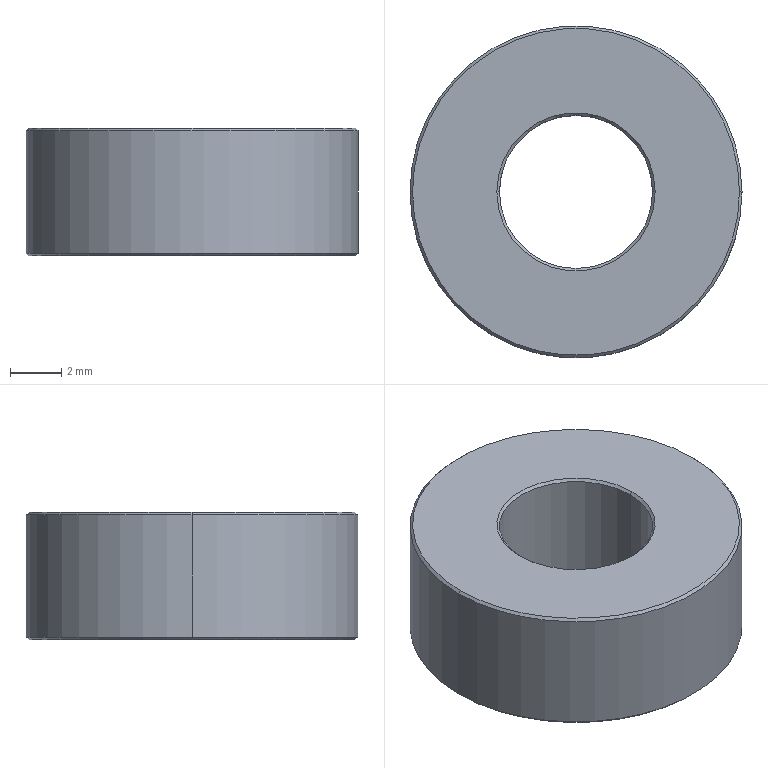Part | SolidWorks | features Chamfer 1, Extrusion 1 | 1 solid | 14 faces | box 13 x 13 x 5 mm | volume 521.693 mm3 | cone 8 | cylinder 4 | plane 2 | commonest cylinder face diameters 6 x2 13 x2
STEP:
#1=CARTESIAN_POINT('',(-6.4,0.,0.));
#2=VERTEX_POINT('',#1);
#3=CARTESIAN_POINT('',(6.4,0.,0.));
#4=VERTEX_POINT('',#3);
#5=CARTESIAN_POINT('',(0.,0.,0.));
#6=DIRECTION('',(0.,0.,-1.));
#7=DIRECTION('',(1.,0.,0.));
#8=AXIS2_PLACEMENT_3D('',#5,#6,#7);
#9=CIRCLE('',#8,6.4);
#10=EDGE_CURVE('',#2,#4,#9,.T.);
#11=ORIENTED_EDGE('',*,*,#10,.F.);
#12=CARTESIAN_POINT('',(-6.5,0.,0.1));
#13=VERTEX_POINT('',#12);
#14=CARTESIAN_POINT('',(-6.5,0.,0.1));
#15=DIRECTION('',(-0.7071,0.,0.7071));
#16=VECTOR('',#15,1000.);
#17=LINE('',#14,#16);
#18=EDGE_CURVE('',#2,#13,#17,.T.);
#19=ORIENTED_EDGE('',*,*,#18,.T.);
#20=CARTESIAN_POINT('',(6.5,0.,0.1));
#21=VERTEX_POINT('',#20);
#22=CARTESIAN_POINT('',(0.,0.,0.1));
#23=DIRECTION('',(0.,0.,1.));
#24=DIRECTION('',(1.,0.,0.));
#25=AXIS2_PLACEMENT_3D('',#22,#23,#24);
#26=CIRCLE('',#25,6.5);
#27=EDGE_CURVE('',#21,#13,#26,.T.);
#28=ORIENTED_EDGE('',*,*,#27,.F.);
#29=CARTESIAN_POINT('',(6.5,0.,0.1));
#30=DIRECTION('',(0.7071,0.,0.7071));
#31=VECTOR('',#30,1000.);
#32=LINE('',#29,#31);
#33=EDGE_CURVE('',#4,#21,#32,.T.);
#34=ORIENTED_EDGE('',*,*,#33,.F.);
#35=EDGE_LOOP('',(#11,#19,#28,#34));
#36=FACE_OUTER_BOUND('',#35,.T.);
#37=CARTESIAN_POINT('',(0.,0.,0.1));
#38=DIRECTION('',(0.,0.,1.));
#39=DIRECTION('',(1.,0.,0.));
#40=AXIS2_PLACEMENT_3D('',#37,#38,#39);
#41=CONICAL_SURFACE('',#40,6.5,0.7854);
#42=ADVANCED_FACE('',(#36),#41,.T.);
#43=CARTESIAN_POINT('',(3.,0.,0.1));
#44=VERTEX_POINT('',#43);
#45=CARTESIAN_POINT('',(-3.,0.,0.1));
#46=VERTEX_POINT('',#45);
#47=CARTESIAN_POINT('',(0.,0.,0.1));
#48=DIRECTION('',(0.,0.,-1.));
#49=DIRECTION('',(1.,0.,0.));
#50=AXIS2_PLACEMENT_3D('',#47,#48,#49);
#51=CIRCLE('',#50,3.);
#52=EDGE_CURVE('',#44,#46,#51,.T.);
#53=ORIENTED_EDGE('',*,*,#52,.F.);
#54=CARTESIAN_POINT('',(3.1,0.,0.));
#55=VERTEX_POINT('',#54);
#56=CARTESIAN_POINT('',(3.1,0.,0.));
#57=DIRECTION('',(0.7071,0.,-0.7071));
#58=VECTOR('',#57,1000.);
#59=LINE('',#56,#58);
#60=EDGE_CURVE('',#44,#55,#59,.T.);
#61=ORIENTED_EDGE('',*,*,#60,.T.);
#62=CARTESIAN_POINT('',(-3.1,0.,0.));
#63=VERTEX_POINT('',#62);
#64=CARTESIAN_POINT('',(0.,0.,0.));
#65=DIRECTION('',(0.,0.,1.));
#66=DIRECTION('',(1.,0.,0.));
#67=AXIS2_PLACEMENT_3D('',#64,#65,#66);
#68=CIRCLE('',#67,3.1);
#69=EDGE_CURVE('',#63,#55,#68,.T.);
#70=ORIENTED_EDGE('',*,*,#69,.F.);
#71=CARTESIAN_POINT('',(-3.1,0.,0.));
#72=DIRECTION('',(-0.7071,0.,-0.7071));
#73=VECTOR('',#72,1000.);
#74=LINE('',#71,#73);
#75=EDGE_CURVE('',#46,#63,#74,.T.);
#76=ORIENTED_EDGE('',*,*,#75,.F.);
#77=EDGE_LOOP('',(#53,#61,#70,#76));
#78=FACE_OUTER_BOUND('',#77,.T.);
#79=CARTESIAN_POINT('',(0.,0.,0.));
#80=DIRECTION('',(0.,0.,-1.));
#81=DIRECTION('',(-1.,0.,0.));
#82=AXIS2_PLACEMENT_3D('',#79,#80,#81);
#83=CONICAL_SURFACE('',#82,3.1,0.7854);
#84=ADVANCED_FACE('',(#78),#83,.F.);
#85=CARTESIAN_POINT('',(6.4,0.,5.));
#86=VERTEX_POINT('',#85);
#87=CARTESIAN_POINT('',(-6.4,0.,5.));
#88=VERTEX_POINT('',#87);
#89=CARTESIAN_POINT('',(0.,0.,5.));
#90=DIRECTION('',(0.,0.,1.));
#91=DIRECTION('',(1.,0.,0.));
#92=AXIS2_PLACEMENT_3D('',#89,#90,#91);
#93=CIRCLE('',#92,6.4);
#94=EDGE_CURVE('',#86,#88,#93,.T.);
#95=ORIENTED_EDGE('',*,*,#94,.F.);
#96=CARTESIAN_POINT('',(6.5,0.,4.9));
#97=VERTEX_POINT('',#96);
#98=CARTESIAN_POINT('',(6.4,0.,5.));
#99=DIRECTION('',(0.7071,0.,-0.7071));
#100=VECTOR('',#99,1000.);
#101=LINE('',#98,#100);
#102=EDGE_CURVE('',#86,#97,#101,.T.);
#103=ORIENTED_EDGE('',*,*,#102,.T.);
#104=CARTESIAN_POINT('',(-6.5,0.,4.9));
#105=VERTEX_POINT('',#104);
#106=CARTESIAN_POINT('',(0.,0.,4.9));
#107=DIRECTION('',(0.,0.,-1.));
#108=DIRECTION('',(1.,0.,0.));
#109=AXIS2_PLACEMENT_3D('',#106,#107,#108);
#110=CIRCLE('',#109,6.5);
#111=EDGE_CURVE('',#105,#97,#110,.T.);
#112=ORIENTED_EDGE('',*,*,#111,.F.);
#113=CARTESIAN_POINT('',(-6.4,0.,5.));
#114=DIRECTION('',(-0.7071,0.,-0.7071));
#115=VECTOR('',#114,1000.);
#116=LINE('',#113,#115);
#117=EDGE_CURVE('',#88,#105,#116,.T.);
#118=ORIENTED_EDGE('',*,*,#117,.F.);
#119=EDGE_LOOP('',(#95,#103,#112,#118));
#120=FACE_OUTER_BOUND('',#119,.T.);
#121=CARTESIAN_POINT('',(0.,0.,5.));
#122=DIRECTION('',(0.,0.,-1.));
#123=DIRECTION('',(-1.,0.,0.));
#124=AXIS2_PLACEMENT_3D('',#121,#122,#123);
#125=CONICAL_SURFACE('',#124,6.4,0.7854);
#126=ADVANCED_FACE('',(#120),#125,.T.);
#127=CARTESIAN_POINT('',(-3.,0.,4.9));
#128=VERTEX_POINT('',#127);
#129=CARTESIAN_POINT('',(3.,0.,4.9));
#130=VERTEX_POINT('',#129);
#131=CARTESIAN_POINT('',(0.,0.,4.9));
#132=DIRECTION('',(0.,0.,1.));
#133=DIRECTION('',(1.,0.,0.));
#134=AXIS2_PLACEMENT_3D('',#131,#132,#133);
#135=CIRCLE('',#134,3.);
#136=EDGE_CURVE('',#128,#130,#135,.T.);
#137=ORIENTED_EDGE('',*,*,#136,.F.);
#138=CARTESIAN_POINT('',(-3.1,0.,5.));
#139=VERTEX_POINT('',#138);
#140=CARTESIAN_POINT('',(-3.,0.,4.9));
#141=DIRECTION('',(-0.7071,0.,0.7071));
#142=VECTOR('',#141,1000.);
#143=LINE('',#140,#142);
#144=EDGE_CURVE('',#128,#139,#143,.T.);
#145=ORIENTED_EDGE('',*,*,#144,.T.);
#146=CARTESIAN_POINT('',(3.1,0.,5.));
#147=VERTEX_POINT('',#146);
#148=CARTESIAN_POINT('',(0.,0.,5.));
#149=DIRECTION('',(0.,0.,-1.));
#150=DIRECTION('',(1.,0.,0.));
#151=AXIS2_PLACEMENT_3D('',#148,#149,#150);
#152=CIRCLE('',#151,3.1);
#153=EDGE_CURVE('',#147,#139,#152,.T.);
#154=ORIENTED_EDGE('',*,*,#153,.F.);
#155=CARTESIAN_POINT('',(3.,0.,4.9));
#156=DIRECTION('',(0.7071,0.,0.7071));
#157=VECTOR('',#156,1000.);
#158=LINE('',#155,#157);
#159=EDGE_CURVE('',#130,#147,#158,.T.);
#160=ORIENTED_EDGE('',*,*,#159,.F.);
#161=EDGE_LOOP('',(#137,#145,#154,#160));
#162=FACE_OUTER_BOUND('',#161,.T.);
#163=CARTESIAN_POINT('',(0.,0.,4.9));
#164=DIRECTION('',(0.,0.,1.));
#165=DIRECTION('',(1.,0.,0.));
#166=AXIS2_PLACEMENT_3D('',#163,#164,#165);
#167=CONICAL_SURFACE('',#166,3.,0.7854);
#168=ADVANCED_FACE('',(#162),#167,.F.);
#169=ORIENTED_EDGE('',*,*,#136,.T.);
#170=CARTESIAN_POINT('',(3.,0.,5.));
#171=DIRECTION('',(0.,0.,-1.));
#172=VECTOR('',#171,1000.);
#173=LINE('',#170,#172);
#174=EDGE_CURVE('',#130,#44,#173,.T.);
#175=ORIENTED_EDGE('',*,*,#174,.T.);
#176=ORIENTED_EDGE('',*,*,#52,.T.);
#177=CARTESIAN_POINT('',(-3.,0.,5.));
#178=DIRECTION('',(0.,0.,-1.));
#179=VECTOR('',#178,1000.);
#180=LINE('',#177,#179);
#181=EDGE_CURVE('',#128,#46,#180,.T.);
#182=ORIENTED_EDGE('',*,*,#181,.F.);
#183=EDGE_LOOP('',(#169,#175,#176,#182));
#184=FACE_OUTER_BOUND('',#183,.T.);
#185=CARTESIAN_POINT('',(0.,0.,5.));
#186=DIRECTION('',(0.,0.,-1.));
#187=DIRECTION('',(-1.,0.,0.));
#188=AXIS2_PLACEMENT_3D('',#185,#186,#187);
#189=CYLINDRICAL_SURFACE('',#188,3.);
#190=ADVANCED_FACE('',(#184),#189,.F.);
#191=ORIENTED_EDGE('',*,*,#111,.T.);
#192=CARTESIAN_POINT('',(6.5,0.,5.));
#193=DIRECTION('',(0.,0.,-1.));
#194=VECTOR('',#193,1000.);
#195=LINE('',#192,#194);
#196=EDGE_CURVE('',#97,#21,#195,.T.);
#197=ORIENTED_EDGE('',*,*,#196,.T.);
#198=ORIENTED_EDGE('',*,*,#27,.T.);
#199=CARTESIAN_POINT('',(-6.5,0.,5.));
#200=DIRECTION('',(0.,0.,-1.));
#201=VECTOR('',#200,1000.);
#202=LINE('',#199,#201);
#203=EDGE_CURVE('',#105,#13,#202,.T.);
#204=ORIENTED_EDGE('',*,*,#203,.F.);
#205=EDGE_LOOP('',(#191,#197,#198,#204));
#206=FACE_OUTER_BOUND('',#205,.T.);
#207=CARTESIAN_POINT('',(0.,0.,5.));
#208=DIRECTION('',(0.,0.,-1.));
#209=DIRECTION('',(-1.,0.,0.));
#210=AXIS2_PLACEMENT_3D('',#207,#208,#209);
#211=CYLINDRICAL_SURFACE('',#210,6.5);
#212=ADVANCED_FACE('',(#206),#211,.T.);
#213=ORIENTED_EDGE('',*,*,#153,.T.);
#214=CARTESIAN_POINT('',(0.,0.,5.));
#215=DIRECTION('',(0.,0.,-1.));
#216=DIRECTION('',(1.,0.,0.));
#217=AXIS2_PLACEMENT_3D('',#214,#215,#216);
#218=CIRCLE('',#217,3.1);
#219=EDGE_CURVE('',#139,#147,#218,.T.);
#220=ORIENTED_EDGE('',*,*,#219,.T.);
#221=EDGE_LOOP('',(#213,#220));
#222=FACE_BOUND('',#221,.T.);
#223=CARTESIAN_POINT('',(0.,0.,5.));
#224=DIRECTION('',(0.,0.,1.));
#225=DIRECTION('',(1.,0.,0.));
#226=AXIS2_PLACEMENT_3D('',#223,#224,#225);
#227=CIRCLE('',#226,6.4);
#228=EDGE_CURVE('',#88,#86,#227,.T.);
#229=ORIENTED_EDGE('',*,*,#228,.T.);
#230=ORIENTED_EDGE('',*,*,#94,.T.);
#231=EDGE_LOOP('',(#229,#230));
#232=FACE_OUTER_BOUND('',#231,.T.);
#233=CARTESIAN_POINT('',(0.,0.,5.));
#234=DIRECTION('',(0.,0.,1.));
#235=DIRECTION('',(1.,0.,0.));
#236=AXIS2_PLACEMENT_3D('',#233,#234,#235);
#237=PLANE('',#236);
#238=ADVANCED_FACE('',(#222,#232),#237,.T.);
#239=ORIENTED_EDGE('',*,*,#69,.T.);
#240=CARTESIAN_POINT('',(0.,0.,0.));
#241=DIRECTION('',(0.,0.,1.));
#242=DIRECTION('',(1.,0.,0.));
#243=AXIS2_PLACEMENT_3D('',#240,#241,#242);
#244=CIRCLE('',#243,3.1);
#245=EDGE_CURVE('',#55,#63,#244,.T.);
#246=ORIENTED_EDGE('',*,*,#245,.T.);
#247=EDGE_LOOP('',(#239,#246));
#248=FACE_BOUND('',#247,.T.);
#249=CARTESIAN_POINT('',(0.,0.,0.));
#250=DIRECTION('',(0.,0.,-1.));
#251=DIRECTION('',(1.,0.,0.));
#252=AXIS2_PLACEMENT_3D('',#249,#250,#251);
#253=CIRCLE('',#252,6.4);
#254=EDGE_CURVE('',#4,#2,#253,.T.);
#255=ORIENTED_EDGE('',*,*,#254,.T.);
#256=ORIENTED_EDGE('',*,*,#10,.T.);
#257=EDGE_LOOP('',(#255,#256));
#258=FACE_OUTER_BOUND('',#257,.T.);
#259=CARTESIAN_POINT('',(0.,0.,0.));
#260=DIRECTION('',(0.,0.,1.));
#261=DIRECTION('',(1.,0.,0.));
#262=AXIS2_PLACEMENT_3D('',#259,#260,#261);
#263=PLANE('',#262);
#264=ADVANCED_FACE('',(#248,#258),#263,.F.);
#265=ORIENTED_EDGE('',*,*,#196,.F.);
#266=CARTESIAN_POINT('',(0.,0.,4.9));
#267=DIRECTION('',(0.,0.,-1.));
#268=DIRECTION('',(1.,0.,0.));
#269=AXIS2_PLACEMENT_3D('',#266,#267,#268);
#270=CIRCLE('',#269,6.5);
#271=EDGE_CURVE('',#97,#105,#270,.T.);
#272=ORIENTED_EDGE('',*,*,#271,.T.);
#273=ORIENTED_EDGE('',*,*,#203,.T.);
#274=CARTESIAN_POINT('',(0.,0.,0.1));
#275=DIRECTION('',(0.,0.,1.));
#276=DIRECTION('',(1.,0.,0.));
#277=AXIS2_PLACEMENT_3D('',#274,#275,#276);
#278=CIRCLE('',#277,6.5);
#279=EDGE_CURVE('',#13,#21,#278,.T.);
#280=ORIENTED_EDGE('',*,*,#279,.T.);
#281=EDGE_LOOP('',(#265,#272,#273,#280));
#282=FACE_OUTER_BOUND('',#281,.T.);
#283=CARTESIAN_POINT('',(0.,0.,5.));
#284=DIRECTION('',(0.,0.,-1.));
#285=DIRECTION('',(-1.,0.,0.));
#286=AXIS2_PLACEMENT_3D('',#283,#284,#285);
#287=CYLINDRICAL_SURFACE('',#286,6.5);
#288=ADVANCED_FACE('',(#282),#287,.T.);
#289=ORIENTED_EDGE('',*,*,#174,.F.);
#290=CARTESIAN_POINT('',(0.,0.,4.9));
#291=DIRECTION('',(0.,0.,1.));
#292=DIRECTION('',(1.,0.,0.));
#293=AXIS2_PLACEMENT_3D('',#290,#291,#292);
#294=CIRCLE('',#293,3.);
#295=EDGE_CURVE('',#130,#128,#294,.T.);
#296=ORIENTED_EDGE('',*,*,#295,.T.);
#297=ORIENTED_EDGE('',*,*,#181,.T.);
#298=CARTESIAN_POINT('',(0.,0.,0.1));
#299=DIRECTION('',(0.,0.,-1.));
#300=DIRECTION('',(1.,0.,0.));
#301=AXIS2_PLACEMENT_3D('',#298,#299,#300);
#302=CIRCLE('',#301,3.);
#303=EDGE_CURVE('',#46,#44,#302,.T.);
#304=ORIENTED_EDGE('',*,*,#303,.T.);
#305=EDGE_LOOP('',(#289,#296,#297,#304));
#306=FACE_OUTER_BOUND('',#305,.T.);
#307=CARTESIAN_POINT('',(0.,0.,5.));
#308=DIRECTION('',(0.,0.,-1.));
#309=DIRECTION('',(-1.,0.,0.));
#310=AXIS2_PLACEMENT_3D('',#307,#308,#309);
#311=CYLINDRICAL_SURFACE('',#310,3.);
#312=ADVANCED_FACE('',(#306),#311,.F.);
#313=ORIENTED_EDGE('',*,*,#144,.F.);
#314=ORIENTED_EDGE('',*,*,#295,.F.);
#315=ORIENTED_EDGE('',*,*,#159,.T.);
#316=ORIENTED_EDGE('',*,*,#219,.F.);
#317=EDGE_LOOP('',(#313,#314,#315,#316));
#318=FACE_OUTER_BOUND('',#317,.T.);
#319=CARTESIAN_POINT('',(0.,0.,4.9));
#320=DIRECTION('',(0.,0.,1.));
#321=DIRECTION('',(1.,0.,0.));
#322=AXIS2_PLACEMENT_3D('',#319,#320,#321);
#323=CONICAL_SURFACE('',#322,3.,0.7854);
#324=ADVANCED_FACE('',(#318),#323,.F.);
#325=ORIENTED_EDGE('',*,*,#102,.F.);
#326=ORIENTED_EDGE('',*,*,#228,.F.);
#327=ORIENTED_EDGE('',*,*,#117,.T.);
#328=ORIENTED_EDGE('',*,*,#271,.F.);
#329=EDGE_LOOP('',(#325,#326,#327,#328));
#330=FACE_OUTER_BOUND('',#329,.T.);
#331=CARTESIAN_POINT('',(0.,0.,5.));
#332=DIRECTION('',(0.,0.,-1.));
#333=DIRECTION('',(-1.,0.,0.));
#334=AXIS2_PLACEMENT_3D('',#331,#332,#333);
#335=CONICAL_SURFACE('',#334,6.4,0.7854);
#336=ADVANCED_FACE('',(#330),#335,.T.);
#337=ORIENTED_EDGE('',*,*,#60,.F.);
#338=ORIENTED_EDGE('',*,*,#303,.F.);
#339=ORIENTED_EDGE('',*,*,#75,.T.);
#340=ORIENTED_EDGE('',*,*,#245,.F.);
#341=EDGE_LOOP('',(#337,#338,#339,#340));
#342=FACE_OUTER_BOUND('',#341,.T.);
#343=CARTESIAN_POINT('',(0.,0.,0.));
#344=DIRECTION('',(0.,0.,-1.));
#345=DIRECTION('',(-1.,0.,0.));
#346=AXIS2_PLACEMENT_3D('',#343,#344,#345);
#347=CONICAL_SURFACE('',#346,3.1,0.7854);
#348=ADVANCED_FACE('',(#342),#347,.F.);
#349=ORIENTED_EDGE('',*,*,#18,.F.);
#350=ORIENTED_EDGE('',*,*,#254,.F.);
#351=ORIENTED_EDGE('',*,*,#33,.T.);
#352=ORIENTED_EDGE('',*,*,#279,.F.);
#353=EDGE_LOOP('',(#349,#350,#351,#352));
#354=FACE_OUTER_BOUND('',#353,.T.);
#355=CARTESIAN_POINT('',(0.,0.,0.1));
#356=DIRECTION('',(0.,0.,1.));
#357=DIRECTION('',(1.,0.,0.));
#358=AXIS2_PLACEMENT_3D('',#355,#356,#357);
#359=CONICAL_SURFACE('',#358,6.5,0.7854);
#360=ADVANCED_FACE('',(#354),#359,.T.);
#361=CLOSED_SHELL('',(#42,#84,#126,#168,#190,#212,#238,#264,#288,#312,#324,#336,#348,#360));
#362=MANIFOLD_SOLID_BREP('',#361);
#363=CARTESIAN_POINT('',(0.,0.,0.));
#364=DIRECTION('',(0.,0.,1.));
#365=DIRECTION('',(1.,0.,0.));
#366=AXIS2_PLACEMENT_3D('',#363,#364,#365);
#367=(LENGTH_UNIT()NAMED_UNIT(*)SI_UNIT(.MILLI.,.METRE.));
#368=UNCERTAINTY_MEASURE_WITH_UNIT(LENGTH_MEASURE(0.00001),#367,'','');
#369=(NAMED_UNIT(*)PLANE_ANGLE_UNIT()SI_UNIT($,.RADIAN.));
#370=(NAMED_UNIT(*)SI_UNIT($,.STERADIAN.)SOLID_ANGLE_UNIT());
#371=(GEOMETRIC_REPRESENTATION_CONTEXT(3)GLOBAL_UNCERTAINTY_ASSIGNED_CONTEXT((#368))GLOBAL_UNIT_ASSIGNED_CONTEXT((#367,#369,#370))REPRESENTATION_CONTEXT('',''));
#372=ADVANCED_BREP_SHAPE_REPRESENTATION('',(#362,#366),#371);